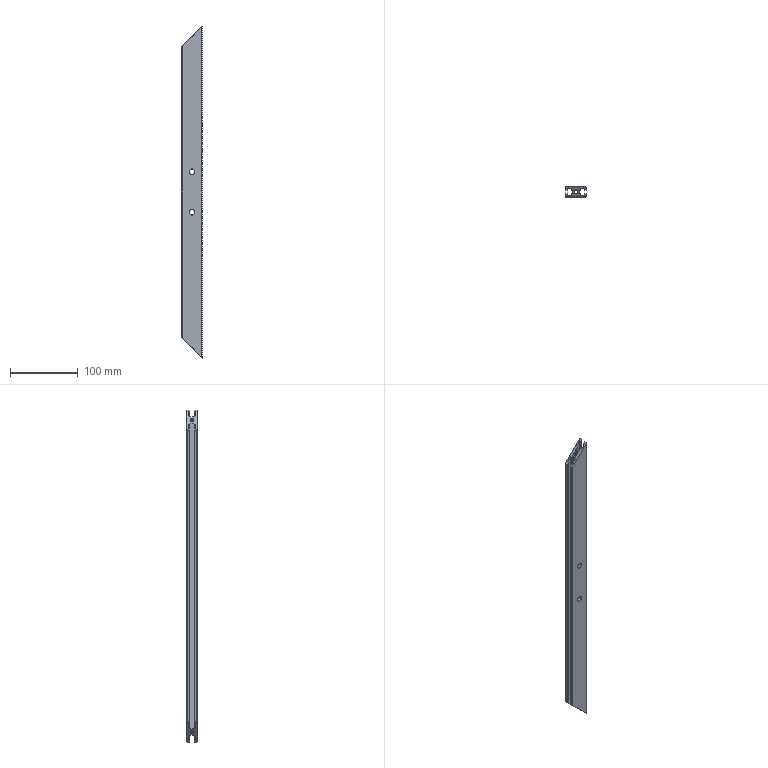Part | NX | features BREP 1 | 1 solid | 127 faces | box 30 x 15 x 491.9 mm | volume 109845 mm3 | cylinder 65 | plane 54 | cone 8 | commonest cylinder face diameters 5 x23 1 x18 3.3 x16 2 x4 8.5 x4